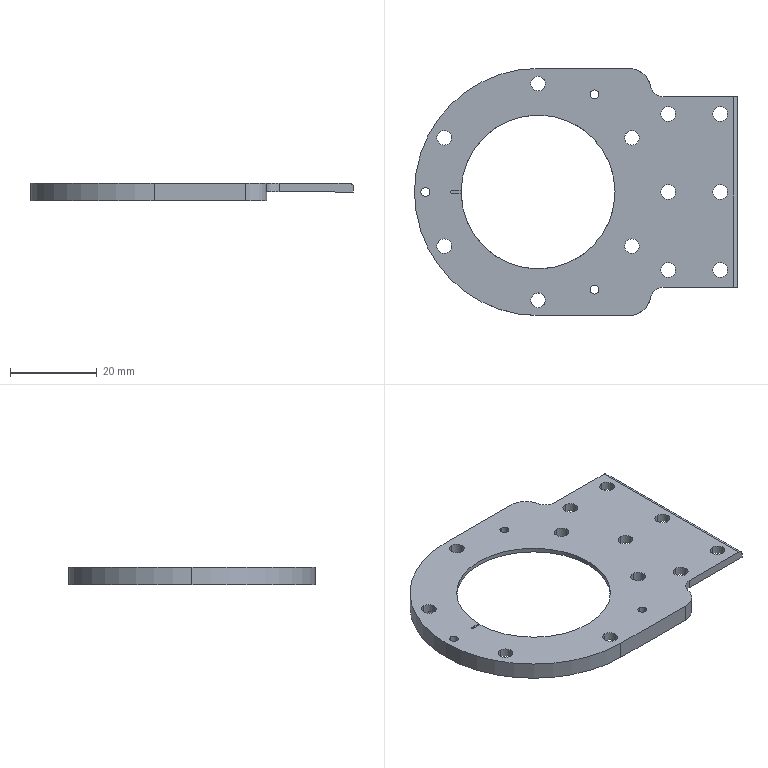NC program | NX | posted with a generic post | part box 74.5 x 57 x 4 mm
Lines 1 to 1634 of 1908, first 1478 of 1622 lines:
N10 G17 G21 G94 G90
(FLOOR_WALL_COPY , TOOL : D80)
N12 T19 M6
N14 G54
N16 G17 G0 G90 X-43. Y0. S5000 M3
N18 G43 Z30. H19
N20 Z3.
N22 G94 G1 Z0. F1200.
N24 X-40.
N26 X114.5
N28 X117.5
N30 Z3.
N32 G0 Z30.
N34 M5
(FLOOR_WALL_1 , TOOL : D4)
N36 T11 M6
N38 G54
N40 G17 G0 G90 X-3.5 Y-1.097 S9500 M3
N42 G43 Z30. H11
N44 Z0.62
N46 G94 G1 Z-0.38 F1000.
N48 X-2.2 Y-0.346
N50 G3 X-2. Y0. R0.4
N52 G1 Y24. F2500.
N54 X17.142
N56 G3 X17.95 Y24.411 R1.
N58 G1 X17.958 Y24.405
N60 G3 X17.9 Y23.5 R7.1
N62 G1 Y-23.5
N64 G3 X17.958 Y-24.405 R7.1
N66 G1 X17.95 Y-24.411
N68 G3 X17.142 Y-24. R1.
N70 G1 X-2.
N72 Y0.
N74 X0.4
N76 Y21.6
N78 X15.5
N80 Y-21.6
N82 X0.4
N84 Y0.
N86 X2.8
N88 Y19.2
N90 X13.1
N92 Y-19.2
N94 X2.8
N96 Y0.
N98 X5.2
N100 Y16.8
N102 X10.7
N104 Y-16.8
N106 X5.2
N108 Y0.
N110 X7.6
N112 Y14.4
N114 X8.3
N116 Y-14.4
N118 X7.6
N120 Y0.
N122 G3 X7.4 Y0.346 R0.4
N124 G1 Z0.62
N126 G0 X-3.5 Y-1.097 Z0.24
N128 G1 Z-0.76 F1000.
N130 X-2.2 Y-0.346
N132 G3 X-2. Y0. R0.4
N134 G1 Y24. F2500.
N136 X17.142
N138 G3 X17.95 Y24.411 R1.
N140 G1 X17.958 Y24.405
N142 G3 X17.9 Y23.5 R7.1
N144 G1 Y-23.5
N146 G3 X17.958 Y-24.405 R7.1
N148 G1 X17.95 Y-24.411
N150 G3 X17.142 Y-24. R1.
N152 G1 X-2.
N154 Y0.
N156 X0.4
N158 Y21.6
N160 X15.5
N162 Y-21.6
N164 X0.4
N166 Y0.
N168 X2.8
N170 Y19.2
N172 X13.1
N174 Y-19.2
N176 X2.8
N178 Y0.
N180 X5.2
N182 Y16.8
N184 X10.7
N186 Y-16.8
N188 X5.2
N190 Y0.
N192 X7.6
N194 Y14.4
N196 X8.3
N198 Y-14.4
N200 X7.6
N202 Y0.
N204 G3 X7.4 Y0.346 R0.4
N206 G1 Z0.24
N208 G0 X-3.5 Y-1.097 Z-0.14
N210 G1 Z-1.14 F1000.
N212 X-2.2 Y-0.346
N214 G3 X-2. Y0. R0.4
N216 G1 Y24. F2500.
N218 X17.142
N220 G3 X17.95 Y24.411 R1.
N222 G1 X17.958 Y24.405
N224 G3 X17.9 Y23.5 R7.1
N226 G1 Y-23.5
N228 G3 X17.958 Y-24.405 R7.1
N230 G1 X17.95 Y-24.411
N232 G3 X17.142 Y-24. R1.
N234 G1 X-2.
N236 Y0.
N238 X0.4
N240 Y21.6
N242 X15.5
N244 Y-21.6
N246 X0.4
N248 Y0.
N250 X2.8
N252 Y19.2
N254 X13.1
N256 Y-19.2
N258 X2.8
N260 Y0.
N262 X5.2
N264 Y16.8
N266 X10.7
N268 Y-16.8
N270 X5.2
N272 Y0.
N274 X7.6
N276 Y14.4
N278 X8.3
N280 Y-14.4
N282 X7.6
N284 Y0.
N286 G3 X7.4 Y0.346 R0.4
N288 G1 Z-0.14
N290 G0 X-3.5 Y-1.097 Z-0.52
N292 G1 Z-1.52 F1000.
N294 X-2.2 Y-0.346
N296 G3 X-2. Y0. R0.4
N298 G1 Y24. F2500.
N300 X17.142
N302 G3 X17.95 Y24.411 R1.
N304 G1 X17.958 Y24.405
N306 G3 X17.9 Y23.5 R7.1
N308 G1 Y-23.5
N310 G3 X17.958 Y-24.405 R7.1
N312 G1 X17.95 Y-24.411
N314 G3 X17.142 Y-24. R1.
N316 G1 X-2.
N318 Y0.
N320 X0.4
N322 Y21.6
N324 X15.5
N326 Y-21.6
N328 X0.4
N330 Y0.
N332 X2.8
N334 Y19.2
N336 X13.1
N338 Y-19.2
N340 X2.8
N342 Y0.
N344 X5.2
N346 Y16.8
N348 X10.7
N350 Y-16.8
N352 X5.2
N354 Y0.
N356 X7.6
N358 Y14.4
N360 X8.3
N362 Y-14.4
N364 X7.6
N366 Y0.
N368 G3 X7.4 Y0.346 R0.4
N370 G1 Z-0.52
N372 G0 X-3.5 Y-1.097 Z-0.9
N374 G1 Z-1.9 F1000.
N376 X-2.2 Y-0.346
N378 G3 X-2. Y0. R0.4
N380 G1 Y24. F2500.
N382 X17.142
N384 G3 X17.95 Y24.411 R1.
N386 G1 X17.958 Y24.405
N388 G3 X17.9 Y23.5 R7.1
N390 G1 Y-23.5
N392 G3 X17.958 Y-24.405 R7.1
N394 G1 X17.95 Y-24.411
N396 G3 X17.142 Y-24. R1.
N398 G1 X-2.
N400 Y0.
N402 X0.4
N404 Y21.6
N406 X15.5
N408 Y-21.6
N410 X0.4
N412 Y0.
N414 X2.8
N416 Y19.2
N418 X13.1
N420 Y-19.2
N422 X2.8
N424 Y0.
N426 X5.2
N428 Y16.8
N430 X10.7
N432 Y-16.8
N434 X5.2
N436 Y0.
N438 X7.6
N440 Y14.4
N442 X8.3
N444 Y-14.4
N446 X7.6
N448 Y0.
N450 G3 X7.4 Y0.346 R0.4
N452 G1 Z-0.9
N454 G0 Z30.
(FLOOR_WALL_1_COPY , TOOL : D4)
N456 X47.556 Y-21.217
N458 Z0.62
N460 G1 Z-0.38 F700.
N462 G3 X47.938 Y-21.336 R0.4
N464 X46. Y-22.707 R3.1 F2500.
N466 X43.709 Y-21.277 R3.1
N468 G2 X28.719 Y-12.623 R21.4
N470 G3 X26.335 Y-11.353 R3.1
N472 X26.428 Y-8.654 R3.1
N474 G2 X26.428 Y8.654 R21.4
N476 G3 X26.335 Y11.353 R3.1
N478 X28.719 Y12.623 R3.1
N480 G2 X43.709 Y21.277 R21.4
N482 G3 X46. Y22.707 R3.1
N484 X48.291 Y21.277 R3.1
N486 G2 X63.281 Y12.623 R21.4
N488 G3 X65.665 Y11.353 R3.1
N490 X65.572 Y8.654 R3.1
N492 G2 X65.572 Y-8.654 R21.4
N494 G3 X65.665 Y-11.353 R3.1
N496 X63.281 Y-12.623 R3.1
N498 G2 X48.291 Y-21.277 R21.4
N500 G3 X47.938 Y-21.336 R3.1
N502 G1 X47.407 Y-18.995
N504 G3 X46. Y-19.525 R5.5
N506 X43.966 Y-18.891 R5.5
N508 G2 X30.657 Y-11.207 R19.
N510 G3 X29.091 Y-9.762 R5.5
N512 X28.623 Y-7.684 R5.5
N514 G2 X28.623 Y7.684 R19.
N516 G3 X29.091 Y9.762 R5.5
N518 X30.657 Y11.207 R5.5
N520 G2 X43.966 Y18.891 R19.
N522 G3 X46. Y19.525 R5.5
N524 X48.034 Y18.891 R5.5
N526 G2 X61.343 Y11.207 R19.
N528 G3 X62.909 Y9.762 R5.5
N530 X63.377 Y7.684 R5.5
N532 G2 X63.377 Y-7.684 R19.
N534 G3 X62.909 Y-9.762 R5.5
N536 X61.343 Y-11.207 R5.5
N538 G2 X48.034 Y-18.891 R19.
N540 G3 X47.407 Y-18.995 R5.5
N542 G1 X46.877 Y-16.655
N544 G3 X46. Y-16.907 R7.9
N546 X44.223 Y-16.505 R7.9
N548 G2 X32.595 Y-9.791 R16.6
N550 G3 X31.358 Y-8.454 R7.9
N552 X30.818 Y-6.713 R7.9
N554 G2 X30.818 Y6.713 R16.6
N556 G3 X31.358 Y8.454 R7.9
N558 X32.595 Y9.791 R7.9
N560 G2 X44.223 Y16.505 R16.6
N562 G3 X46. Y16.907 R7.9
N564 X47.777 Y16.505 R7.9
N566 G2 X59.405 Y9.791 R16.6
N568 G3 X60.642 Y8.454 R7.9
N570 X61.182 Y6.713 R7.9
N572 G2 X61.182 Y-6.713 R16.6
N574 G3 X60.642 Y-8.454 R7.9
N576 X59.405 Y-9.791 R7.9
N578 G2 X47.777 Y-16.505 R16.6
N580 G3 X46.877 Y-16.655 R7.9
N582 X46.583 Y-16.926 R0.4
N584 G1 Z0.62
N586 G0 X47.556 Y-21.217 Z0.24
N588 G1 Z-0.76 F700.
N590 G3 X47.938 Y-21.336 R0.4
N592 X46. Y-22.707 R3.1 F2500.
N594 X43.709 Y-21.277 R3.1
N596 G2 X28.719 Y-12.623 R21.4
N598 G3 X26.335 Y-11.353 R3.1
N600 X26.428 Y-8.654 R3.1
N602 G2 X26.428 Y8.654 R21.4
N604 G3 X26.335 Y11.353 R3.1
N606 X28.719 Y12.623 R3.1
N608 G2 X43.709 Y21.277 R21.4
N610 G3 X46. Y22.707 R3.1
N612 X48.291 Y21.277 R3.1
N614 G2 X63.281 Y12.623 R21.4
N616 G3 X65.665 Y11.353 R3.1
N618 X65.572 Y8.654 R3.1
N620 G2 X65.572 Y-8.654 R21.4
N622 G3 X65.665 Y-11.353 R3.1
N624 X63.281 Y-12.623 R3.1
N626 G2 X48.291 Y-21.277 R21.4
N628 G3 X47.938 Y-21.336 R3.1
N630 G1 X47.407 Y-18.995
N632 G3 X46. Y-19.525 R5.5
N634 X43.966 Y-18.891 R5.5
N636 G2 X30.657 Y-11.207 R19.
N638 G3 X29.091 Y-9.762 R5.5
N640 X28.623 Y-7.684 R5.5
N642 G2 X28.623 Y7.684 R19.
N644 G3 X29.091 Y9.762 R5.5
N646 X30.657 Y11.207 R5.5
N648 G2 X43.966 Y18.891 R19.
N650 G3 X46. Y19.525 R5.5
N652 X48.034 Y18.891 R5.5
N654 G2 X61.343 Y11.207 R19.
N656 G3 X62.909 Y9.762 R5.5
N658 X63.377 Y7.684 R5.5
N660 G2 X63.377 Y-7.684 R19.
N662 G3 X62.909 Y-9.762 R5.5
N664 X61.343 Y-11.207 R5.5
N666 G2 X48.034 Y-18.891 R19.
N668 G3 X47.407 Y-18.995 R5.5
N670 G1 X46.877 Y-16.655
N672 G3 X46. Y-16.907 R7.9
N674 X44.223 Y-16.505 R7.9
N676 G2 X32.595 Y-9.791 R16.6
N678 G3 X31.358 Y-8.454 R7.9
N680 X30.818 Y-6.713 R7.9
N682 G2 X30.818 Y6.713 R16.6
N684 G3 X31.358 Y8.454 R7.9
N686 X32.595 Y9.791 R7.9
N688 G2 X44.223 Y16.505 R16.6
N690 G3 X46. Y16.907 R7.9
N692 X47.777 Y16.505 R7.9
N694 G2 X59.405 Y9.791 R16.6
N696 G3 X60.642 Y8.454 R7.9
N698 X61.182 Y6.713 R7.9
N700 G2 X61.182 Y-6.713 R16.6
N702 G3 X60.642 Y-8.454 R7.9
N704 X59.405 Y-9.791 R7.9
N706 G2 X47.777 Y-16.505 R16.6
N708 G3 X46.877 Y-16.655 R7.9
N710 X46.583 Y-16.926 R0.4
N712 G1 Z0.24
N714 G0 X47.556 Y-21.217 Z-0.14
N716 G1 Z-1.14 F700.
N718 G3 X47.938 Y-21.336 R0.4
N720 X46. Y-22.707 R3.1 F2500.
N722 X43.709 Y-21.277 R3.1
N724 G2 X28.719 Y-12.623 R21.4
N726 G3 X26.335 Y-11.353 R3.1
N728 X26.428 Y-8.654 R3.1
N730 G2 X26.428 Y8.654 R21.4
N732 G3 X26.335 Y11.353 R3.1
N734 X28.719 Y12.623 R3.1
N736 G2 X43.709 Y21.277 R21.4
N738 G3 X46. Y22.707 R3.1
N740 X48.291 Y21.277 R3.1
N742 G2 X63.281 Y12.623 R21.4
N744 G3 X65.665 Y11.353 R3.1
N746 X65.572 Y8.654 R3.1
N748 G2 X65.572 Y-8.654 R21.4
N750 G3 X65.665 Y-11.353 R3.1
N752 X63.281 Y-12.623 R3.1
N754 G2 X48.291 Y-21.277 R21.4
N756 G3 X47.938 Y-21.336 R3.1
N758 G1 X47.407 Y-18.995
N760 G3 X46. Y-19.525 R5.5
N762 X43.966 Y-18.891 R5.5
N764 G2 X30.657 Y-11.207 R19.
N766 G3 X29.091 Y-9.762 R5.5
N768 X28.623 Y-7.684 R5.5
N770 G2 X28.623 Y7.684 R19.
N772 G3 X29.091 Y9.762 R5.5
N774 X30.657 Y11.207 R5.5
N776 G2 X43.966 Y18.891 R19.
N778 G3 X46. Y19.525 R5.5
N780 X48.034 Y18.891 R5.5
N782 G2 X61.343 Y11.207 R19.
N784 G3 X62.909 Y9.762 R5.5
N786 X63.377 Y7.684 R5.5
N788 G2 X63.377 Y-7.684 R19.
N790 G3 X62.909 Y-9.762 R5.5
N792 X61.343 Y-11.207 R5.5
N794 G2 X48.034 Y-18.891 R19.
N796 G3 X47.407 Y-18.995 R5.5
N798 G1 X46.877 Y-16.655
N800 G3 X46. Y-16.907 R7.9
N802 X44.223 Y-16.505 R7.9
N804 G2 X32.595 Y-9.791 R16.6
N806 G3 X31.358 Y-8.454 R7.9
N808 X30.818 Y-6.713 R7.9
N810 G2 X30.818 Y6.713 R16.6
N812 G3 X31.358 Y8.454 R7.9
N814 X32.595 Y9.791 R7.9
N816 G2 X44.223 Y16.505 R16.6
N818 G3 X46. Y16.907 R7.9
N820 X47.777 Y16.505 R7.9
N822 G2 X59.405 Y9.791 R16.6
N824 G3 X60.642 Y8.454 R7.9
N826 X61.182 Y6.713 R7.9
N828 G2 X61.182 Y-6.713 R16.6
N830 G3 X60.642 Y-8.454 R7.9
N832 X59.405 Y-9.791 R7.9
N834 G2 X47.777 Y-16.505 R16.6
N836 G3 X46.877 Y-16.655 R7.9
N838 X46.583 Y-16.926 R0.4
N840 G1 Z-0.14
N842 G0 X47.556 Y-21.217 Z-0.52
N844 G1 Z-1.52 F700.
N846 G3 X47.938 Y-21.336 R0.4
N848 X46. Y-22.707 R3.1 F2500.
N850 X43.709 Y-21.277 R3.1
N852 G2 X28.719 Y-12.623 R21.4
N854 G3 X26.335 Y-11.353 R3.1
N856 X26.428 Y-8.654 R3.1
N858 G2 X26.428 Y8.654 R21.4
N860 G3 X26.335 Y11.353 R3.1
N862 X28.719 Y12.623 R3.1
N864 G2 X43.709 Y21.277 R21.4
N866 G3 X46. Y22.707 R3.1
N868 X48.291 Y21.277 R3.1
N870 G2 X63.281 Y12.623 R21.4
N872 G3 X65.665 Y11.353 R3.1
N874 X65.572 Y8.654 R3.1
N876 G2 X65.572 Y-8.654 R21.4
N878 G3 X65.665 Y-11.353 R3.1
N880 X63.281 Y-12.623 R3.1
N882 G2 X48.291 Y-21.277 R21.4
N884 G3 X47.938 Y-21.336 R3.1
N886 G1 X47.407 Y-18.995
N888 G3 X46. Y-19.525 R5.5
N890 X43.966 Y-18.891 R5.5
N892 G2 X30.657 Y-11.207 R19.
N894 G3 X29.091 Y-9.762 R5.5
N896 X28.623 Y-7.684 R5.5
N898 G2 X28.623 Y7.684 R19.
N900 G3 X29.091 Y9.762 R5.5
N902 X30.657 Y11.207 R5.5
N904 G2 X43.966 Y18.891 R19.
N906 G3 X46. Y19.525 R5.5
N908 X48.034 Y18.891 R5.5
N910 G2 X61.343 Y11.207 R19.
N912 G3 X62.909 Y9.762 R5.5
N914 X63.377 Y7.684 R5.5
N916 G2 X63.377 Y-7.684 R19.
N918 G3 X62.909 Y-9.762 R5.5
N920 X61.343 Y-11.207 R5.5
N922 G2 X48.034 Y-18.891 R19.
N924 G3 X47.407 Y-18.995 R5.5
N926 G1 X46.877 Y-16.655
N928 G3 X46. Y-16.907 R7.9
N930 X44.223 Y-16.505 R7.9
N932 G2 X32.595 Y-9.791 R16.6
N934 G3 X31.358 Y-8.454 R7.9
N936 X30.818 Y-6.713 R7.9
N938 G2 X30.818 Y6.713 R16.6
N940 G3 X31.358 Y8.454 R7.9
N942 X32.595 Y9.791 R7.9
N944 G2 X44.223 Y16.505 R16.6
N946 G3 X46. Y16.907 R7.9
N948 X47.777 Y16.505 R7.9
N950 G2 X59.405 Y9.791 R16.6
N952 G3 X60.642 Y8.454 R7.9
N954 X61.182 Y6.713 R7.9
N956 G2 X61.182 Y-6.713 R16.6
N958 G3 X60.642 Y-8.454 R7.9
N960 X59.405 Y-9.791 R7.9
N962 G2 X47.777 Y-16.505 R16.6
N964 G3 X46.877 Y-16.655 R7.9
N966 X46.583 Y-16.926 R0.4
N968 G1 Z-0.52
N970 G0 X47.556 Y-21.217 Z-0.9
N972 G1 Z-1.9 F700.
N974 G3 X47.938 Y-21.336 R0.4
N976 X46. Y-22.707 R3.1 F2500.
N978 X43.709 Y-21.277 R3.1
N980 G2 X28.719 Y-12.623 R21.4
N982 G3 X26.335 Y-11.353 R3.1
N984 X26.428 Y-8.654 R3.1
N986 G2 X26.428 Y8.654 R21.4
N988 G3 X26.335 Y11.353 R3.1
N990 X28.719 Y12.623 R3.1
N992 G2 X43.709 Y21.277 R21.4
N994 G3 X46. Y22.707 R3.1
N996 X48.291 Y21.277 R3.1
N998 G2 X63.281 Y12.623 R21.4
N1000 G3 X65.665 Y11.353 R3.1
N1002 X65.572 Y8.654 R3.1
N1004 G2 X65.572 Y-8.654 R21.4
N1006 G3 X65.665 Y-11.353 R3.1
N1008 X63.281 Y-12.623 R3.1
N1010 G2 X48.291 Y-21.277 R21.4
N1012 G3 X47.938 Y-21.336 R3.1
N1014 G1 X47.407 Y-18.995
N1016 G3 X46. Y-19.525 R5.5
N1018 X43.966 Y-18.891 R5.5
N1020 G2 X30.657 Y-11.207 R19.
N1022 G3 X29.091 Y-9.762 R5.5
N1024 X28.623 Y-7.684 R5.5
N1026 G2 X28.623 Y7.684 R19.
N1028 G3 X29.091 Y9.762 R5.5
N1030 X30.657 Y11.207 R5.5
N1032 G2 X43.966 Y18.891 R19.
N1034 G3 X46. Y19.525 R5.5
N1036 X48.034 Y18.891 R5.5
N1038 G2 X61.343 Y11.207 R19.
N1040 G3 X62.909 Y9.762 R5.5
N1042 X63.377 Y7.684 R5.5
N1044 G2 X63.377 Y-7.684 R19.
N1046 G3 X62.909 Y-9.762 R5.5
N1048 X61.343 Y-11.207 R5.5
N1050 G2 X48.034 Y-18.891 R19.
N1052 G3 X47.407 Y-18.995 R5.5
N1054 G1 X46.877 Y-16.655
N1056 G3 X46. Y-16.907 R7.9
N1058 X44.223 Y-16.505 R7.9
N1060 G2 X32.595 Y-9.791 R16.6
N1062 G3 X31.358 Y-8.454 R7.9
N1064 X30.818 Y-6.713 R7.9
N1066 G2 X30.818 Y6.713 R16.6
N1068 G3 X31.358 Y8.454 R7.9
N1070 X32.595 Y9.791 R7.9
N1072 G2 X44.223 Y16.505 R16.6
N1074 G3 X46. Y16.907 R7.9
N1076 X47.777 Y16.505 R7.9
N1078 G2 X59.405 Y9.791 R16.6
N1080 G3 X60.642 Y8.454 R7.9
N1082 X61.182 Y6.713 R7.9
N1084 G2 X61.182 Y-6.713 R16.6
N1086 G3 X60.642 Y-8.454 R7.9
N1088 X59.405 Y-9.791 R7.9
N1090 G2 X47.777 Y-16.505 R16.6
N1092 G3 X46.877 Y-16.655 R7.9
N1094 X46.583 Y-16.926 R0.4
N1096 G1 Z-0.9
N1098 G0 Z30.
(FLOOR_WALL_1_COPY_COPY , TOOL : D4)
N1100 X46.346 Y17.7
N1102 Z-1.3
N1104 G1 Z-2.3 F700.
N1106 G3 X46. Y17.9 R0.4
N1108 G2 X63.9 Y0. R17.9 F2500.
N1110 X46. Y17.9 R-17.9
N1112 G1 Y15.5
N1114 G2 X61.5 Y0. R15.5
N1116 X46. Y15.5 R-15.5
N1118 G3 X46.346 Y15.7 R0.4
N1120 G1 Z-1.3
N1122 G0 Y17.7 Z-1.6
N1124 G1 Z-2.6 F700.
N1126 G3 X46. Y17.9 R0.4
N1128 G2 X63.9 Y0. R17.9 F2500.
N1130 X46. Y17.9 R-17.9
N1132 G1 Y15.5
N1134 G2 X61.5 Y0. R15.5
N1136 X46. Y15.5 R-15.5
N1138 G3 X46.346 Y15.7 R0.4
N1140 G1 Z-1.6
N1142 G0 Y17.7 Z-1.9
N1144 G1 Z-2.9 F700.
N1146 G3 X46. Y17.9 R0.4
N1148 G2 X63.9 Y0. R17.9 F2500.
N1150 X46. Y17.9 R-17.9
N1152 G1 Y15.5
N1154 G2 X61.5 Y0. R15.5
N1156 X46. Y15.5 R-15.5
N1158 G3 X46.346 Y15.7 R0.4
N1160 G1 Z-1.9
N1162 G0 Z30.
N1164 M5
(FLOOR_WALL_1_COPY_COPY_1 , TOOL : D3)
N1166 T16 M6
N1168 G54
N1170 G17 G0 G90 X67.44 Y12.382 S9500 M3
N1172 G43 Z30. H16
N1174 Z-0.9
N1176 G94 G1 X67.473 Y12.409 Z-0.911 F700.
N1178 X67.448 Y12.388 Z-0.92
N1180 X67.423 Y12.369 Z-0.928
N1182 X67.453 Y12.381 Z-0.937
N1184 X67.483 Y12.392 Z-0.945
N1186 X67.453 Y12.381 Z-0.954
N1188 X67.423 Y12.369 Z-0.962
N1190 X67.448 Y12.388 Z-0.971
N1192 X67.473 Y12.409 Z-0.979
N1194 X67.448 Y12.388 Z-0.988
N1196 X67.423 Y12.369 Z-0.996
N1198 X67.453 Y12.381 Z-1.005
N1200 X67.483 Y12.392 Z-1.013
N1202 X67.453 Y12.381 Z-1.022
N1204 X67.423 Y12.369 Z-1.03
N1206 X67.448 Y12.388 Z-1.039
N1208 X67.473 Y12.409 Z-1.047
N1210 X67.448 Y12.388 Z-1.056
N1212 X67.423 Y12.369 Z-1.064
N1214 X67.453 Y12.381 Z-1.073
N1216 X67.483 Y12.392 Z-1.081
N1218 X67.453 Y12.381 Z-1.09
N1220 X67.423 Y12.369 Z-1.098
N1222 X67.448 Y12.388 Z-1.107
N1224 X67.473 Y12.409 Z-1.115
N1226 X67.448 Y12.388 Z-1.124
N1228 X67.423 Y12.369 Z-1.132
N1230 X67.453 Y12.381 Z-1.141
N1232 X67.483 Y12.392 Z-1.149
N1234 X67.453 Y12.381 Z-1.158
N1236 X67.423 Y12.369 Z-1.166
N1238 X67.448 Y12.388 Z-1.175
N1240 X67.473 Y12.409 Z-1.183
N1242 X67.448 Y12.388 Z-1.192
N1244 X67.423 Y12.369 Z-1.2
N1246 X67.453 Y12.381 Z-1.209
N1248 X67.483 Y12.392 Z-1.217
N1250 X67.453 Y12.381 Z-1.226
N1252 X67.423 Y12.369 Z-1.234
N1254 X67.448 Y12.388 Z-1.243
N1256 X67.473 Y12.409 Z-1.251
N1258 X67.448 Y12.388 Z-1.26
N1260 X67.423 Y12.369 Z-1.268
N1262 X67.453 Y12.381 Z-1.277
N1264 X67.483 Y12.392 Z-1.285
N1266 X67.453 Y12.381 Z-1.294
N1268 X67.423 Y12.369 Z-1.302
N1270 X67.448 Y12.388 Z-1.311
N1272 X67.473 Y12.409 Z-1.32
N1274 X67.448 Y12.388 Z-1.328
N1276 X67.423 Y12.369 Z-1.337
N1278 X67.453 Y12.381 Z-1.345
N1280 X67.483 Y12.392 Z-1.354
N1282 X67.453 Y12.381 Z-1.362
N1284 X67.423 Y12.369 Z-1.371
N1286 X67.448 Y12.388 Z-1.379
N1288 X67.473 Y12.409 Z-1.388
N1290 X67.448 Y12.388 Z-1.396
N1292 X67.423 Y12.369 Z-1.405
N1294 X67.453 Y12.381 Z-1.413
N1296 X67.483 Y12.392 Z-1.422
N1298 X67.453 Y12.381 Z-1.43
N1300 X67.423 Y12.369 Z-1.439
N1302 X67.448 Y12.388 Z-1.447
N1304 X67.473 Y12.409 Z-1.456
N1306 X67.448 Y12.388 Z-1.464
N1308 X67.423 Y12.369 Z-1.473
N1310 X67.453 Y12.381 Z-1.481
N1312 X67.483 Y12.392 Z-1.49
N1314 X67.453 Y12.381 Z-1.498
N1316 X67.423 Y12.369 Z-1.507
N1318 X67.448 Y12.388 Z-1.515
N1320 X67.473 Y12.409 Z-1.524
N1322 X67.448 Y12.388 Z-1.532
N1324 X67.423 Y12.369 Z-1.541
N1326 X67.453 Y12.381 Z-1.549
N1328 X67.483 Y12.392 Z-1.558
N1330 X67.453 Y12.381 Z-1.566
N1332 X67.423 Y12.369 Z-1.575
N1334 X67.448 Y12.388 Z-1.583
N1336 X67.473 Y12.409 Z-1.592
N1338 X67.448 Y12.388 Z-1.6
N1340 X67.423 Y12.369 Z-1.609
N1342 X67.453 Y12.381 Z-1.617
N1344 X67.483 Y12.392 Z-1.626
N1346 X67.453 Y12.381 Z-1.634
N1348 X67.423 Y12.369 Z-1.643
N1350 X67.448 Y12.388 Z-1.651
N1352 X67.473 Y12.409 Z-1.66
N1354 X67.448 Y12.388 Z-1.668
N1356 X67.423 Y12.369 Z-1.677
N1358 X67.453 Y12.381 Z-1.685
N1360 X67.483 Y12.392 Z-1.694
N1362 X67.453 Y12.381 Z-1.702
N1364 X67.423 Y12.369 Z-1.711
N1366 X67.448 Y12.388 Z-1.719
N1368 X67.473 Y12.409 Z-1.728
N1370 X67.448 Y12.388 Z-1.736
N1372 X67.423 Y12.369 Z-1.745
N1374 X67.453 Y12.381 Z-1.753
N1376 X67.483 Y12.392 Z-1.762
N1378 X67.453 Y12.381 Z-1.77
N1380 X67.423 Y12.369 Z-1.779
N1382 X67.448 Y12.388 Z-1.787
N1384 X67.473 Y12.409 Z-1.796
N1386 X67.448 Y12.388 Z-1.804
N1388 X67.423 Y12.369 Z-1.813
N1390 X67.453 Y12.381 Z-1.821
N1392 X67.483 Y12.392 Z-1.83
N1394 X67.453 Y12.381 Z-1.838
N1396 X67.423 Y12.369 Z-1.847
N1398 X67.448 Y12.388 Z-1.855
N1400 X67.473 Y12.409 Z-1.864
N1402 X67.448 Y12.388 Z-1.872
N1404 X67.423 Y12.369 Z-1.881
N1406 X67.453 Y12.381 Z-1.889
N1408 X67.483 Y12.392 Z-1.898
N1410 X67.453 Y12.381 Z-1.906
N1412 X67.423 Y12.369 Z-1.915
N1414 X67.448 Y12.388 Z-1.923
N1416 X67.473 Y12.409 Z-1.932
N1418 X67.448 Y12.388 Z-1.94
N1420 X67.423 Y12.369 Z-1.949
N1422 X67.453 Y12.381 Z-1.957
N1424 X67.483 Y12.392 Z-1.966
N1426 X67.453 Y12.381 Z-1.974
N1428 X67.423 Y12.369 Z-1.983
N1430 X67.448 Y12.388 Z-1.991
N1432 X67.473 Y12.409 Z-2.
N1434 X67.423 Y12.369 F1200.
N1436 X67.483 Y12.392
N1438 Z-1.
N1440 G0 Z30.
N1442 X48.354 Y21.56
N1444 Z-1.
N1446 G1 Z-2. F700.
N1448 G3 X48.127 Y21.756 R0.3
N1450 X48.339 Y21.724 R2.65 F1200.
N1452 G2 X63.644 Y12.888 R21.85
N1454 G3 X66.768 Y11.99 R2.65
N1456 X65.983 Y8.836 R2.65
N1458 G2 X65.983 Y-8.836 R21.85
N1460 G3 X66.768 Y-11.99 R2.65
N1462 X63.644 Y-12.888 R2.65
N1464 G2 X48.339 Y-21.724 R21.85
N1466 G3 X46. Y-23.981 R2.65
N1468 X43.661 Y-21.724 R2.65
N1470 G2 X28.356 Y-12.888 R21.85
N1472 G3 X25.232 Y-11.99 R2.65
N1474 X26.017 Y-8.836 R2.65
N1476 G2 X26.017 Y8.836 R21.85
N1478 G3 X25.232 Y11.99 R2.65
N1480 X28.356 Y12.888 R2.65
N1482 G2 X43.661 Y21.724 R21.85
N1484 G3 X46. Y23.981 R2.65
N1486 X48.127 Y21.756 R2.65
N1488 G1 X47.789 Y19.988
N1490 G3 X48.146 Y19.935 R4.45
N1492 G2 X62.191 Y11.826 R20.05
N1494 G3 X63.982 Y10.382 R4.45
N1496 X64.337 Y8.108 R4.45
N1498 G2 X64.337 Y-8.108 R20.05
N1500 G3 X63.982 Y-10.382 R4.45
N1502 X62.191 Y-11.826 R4.45
N1504 G2 X48.146 Y-19.935 R20.05
N1506 G3 X46. Y-20.764 R4.45
N1508 X43.854 Y-19.935 R4.45
N1510 G2 X29.809 Y-11.826 R20.05
N1512 G3 X28.018 Y-10.382 R4.45
N1514 X27.663 Y-8.108 R4.45
N1516 G2 X27.663 Y8.108 R20.05
N1518 G3 X28.018 Y10.382 R4.45
N1520 X29.809 Y11.826 R4.45
N1522 G2 X43.854 Y19.935 R20.05
N1524 G3 X46. Y20.764 R4.45
N1526 X47.789 Y19.988 R4.45
N1528 G1 X47.452 Y18.22
N1530 G3 X47.954 Y18.145 R6.25
N1532 G2 X60.737 Y10.765 R18.25
N1534 G3 X62.183 Y9.343 R6.25
N1536 X62.691 Y7.381 R6.25
N1538 G2 X62.691 Y-7.381 R18.25
N1540 G3 X62.183 Y-9.343 R6.25
N1542 X60.737 Y-10.765 R6.25
N1544 G2 X47.954 Y-18.145 R18.25
N1546 G3 X46. Y-18.686 R6.25
N1548 X44.046 Y-18.145 R6.25
N1550 G2 X31.263 Y-10.765 R18.25
N1552 G3 X29.817 Y-9.343 R6.25
N1554 X29.309 Y-7.381 R6.25
N1556 G2 X29.309 Y7.38 R18.25
N1558 G3 X29.817 Y9.343 R6.25
N1560 X31.263 Y10.765 R6.25
N1562 G2 X44.046 Y18.145 R18.25
N1564 G3 X46. Y18.686 R6.25
N1566 X47.452 Y18.22 R6.25
N1568 G1 X47.115 Y16.452
N1570 G3 X47.761 Y16.355 R8.05
N1572 G2 X59.284 Y9.703 R16.45
N1574 G3 X60.505 Y8.374 R8.05
N1576 X61.045 Y6.653 R8.05
N1578 G2 X61.045 Y-6.653 R16.45
N1580 G3 X60.505 Y-8.374 R8.05
N1582 X59.284 Y-9.703 R8.05
N1584 G2 X47.761 Y-16.355 R16.45
N1586 G3 X46. Y-16.748 R8.05
N1588 X44.239 Y-16.355 R8.05
N1590 G2 X32.716 Y-9.703 R16.45
N1592 G3 X31.495 Y-8.374 R8.05
N1594 X30.955 Y-6.653 R8.05
N1596 G2 X30.955 Y6.652 R16.45
N1598 G3 X31.495 Y8.374 R8.05
N1600 X32.716 Y9.703 R8.05
N1602 G2 X44.239 Y16.355 R16.45
N1604 G3 X46. Y16.748 R8.05
N1606 X47.115 Y16.452 R8.05
N1608 G1 X46.778 Y14.683
N1610 G3 X47.568 Y14.566 R9.85
N1612 G2 X57.83 Y8.641 R14.65
N1614 G3 X58.873 Y7.432 R9.85
N1616 X59.399 Y5.925 R9.85
N1618 G2 X59.399 Y-5.925 R14.65
N1620 G3 X58.873 Y-7.432 R9.85
N1622 X57.83 Y-8.641 R9.85
N1624 G2 X47.568 Y-14.566 R14.65
N1626 G3 X46. Y-14.865 R9.85
N1628 X44.432 Y-14.566 R9.85
N1630 G2 X34.17 Y-8.641 R14.65
N1632 G3 X33.127 Y-7.432 R9.85
N1634 X32.601 Y-5.925 R9.85
N1636 G2 X32.601 Y5.924 R14.65
N1638 G3 X33.127 Y7.432 R9.85
N1640 X34.17 Y8.641 R9.85
N1642 G2 X44.432 Y14.566 R14.65
N1644 G3 X46. Y14.865 R9.85
N1646 X46.778 Y14.683 R9.85
N1648 X47.061 Y14.782 R0.3
N1650 G1 Z-1.
N1652 G0 X45.997 Y24.759 Z-0.9
N1654 G1 X45.99 Y24.8 Z-0.911 F700.
N1656 X45.995 Y24.769 Z-0.92
N1658 X46. Y24.738 Z-0.928
N1660 X46.005 Y24.769 Z-0.937
N1662 X46.01 Y24.8 Z-0.945
N1664 X46.005 Y24.769 Z-0.954
N1666 X46. Y24.738 Z-0.962
N1668 X45.995 Y24.769 Z-0.971
N1670 X45.99 Y24.8 Z-0.979
N1672 X45.995 Y24.769 Z-0.988
N1674 X46. Y24.738 Z-0.996
N1676 X46.005 Y24.769 Z-1.005
N1678 X46.01 Y24.8 Z-1.013
N1680 X46.005 Y24.769 Z-1.022
N1682 X46. Y24.738 Z-1.03
N1684 X45.995 Y24.769 Z-1.039
N1686 X45.99 Y24.8 Z-1.047
N1688 X45.995 Y24.769 Z-1.056
N1690 X46. Y24.738 Z-1.064
N1692 X46.005 Y24.769 Z-1.073
N1694 X46.01 Y24.8 Z-1.081
N1696 X46.005 Y24.769 Z-1.09
N1698 X46. Y24.738 Z-1.098
N1700 X45.995 Y24.769 Z-1.107
N1702 X45.99 Y24.8 Z-1.115
N1704 X45.995 Y24.769 Z-1.124
N1706 X46. Y24.738 Z-1.132
N1708 X46.005 Y24.769 Z-1.141
N1710 X46.01 Y24.8 Z-1.149
N1712 X46.005 Y24.769 Z-1.158
N1714 X46. Y24.738 Z-1.166
N1716 X45.995 Y24.769 Z-1.175
N1718 X45.99 Y24.8 Z-1.183
N1720 X45.995 Y24.769 Z-1.192
N1722 X46. Y24.738 Z-1.2
N1724 X46.005 Y24.769 Z-1.209
N1726 X46.01 Y24.8 Z-1.217
N1728 X46.005 Y24.769 Z-1.226
N1730 X46. Y24.738 Z-1.234
N1732 X45.995 Y24.769 Z-1.243
N1734 X45.99 Y24.8 Z-1.251
N1736 X45.995 Y24.769 Z-1.26
N1738 X46. Y24.738 Z-1.268
N1740 X46.005 Y24.769 Z-1.277
N1742 X46.01 Y24.8 Z-1.285
N1744 X46.005 Y24.769 Z-1.294
N1746 X46. Y24.738 Z-1.302
N1748 X45.995 Y24.769 Z-1.311
N1750 X45.99 Y24.8 Z-1.32
N1752 X45.995 Y24.769 Z-1.328
N1754 X46. Y24.738 Z-1.337
N1756 X46.005 Y24.769 Z-1.345
N1758 X46.01 Y24.8 Z-1.354
N1760 X46.005 Y24.769 Z-1.362
N1762 X46. Y24.738 Z-1.371
N1764 X45.995 Y24.769 Z-1.379
N1766 X45.99 Y24.8 Z-1.388
N1768 X45.995 Y24.769 Z-1.396
N1770 X46. Y24.738 Z-1.405
N1772 X46.005 Y24.769 Z-1.413
N1774 X46.01 Y24.8 Z-1.422
N1776 X46.005 Y24.769 Z-1.43
N1778 X46. Y24.738 Z-1.439
N1780 X45.995 Y24.769 Z-1.447
N1782 X45.99 Y24.8 Z-1.456
N1784 X45.995 Y24.769 Z-1.464
N1786 X46. Y24.738 Z-1.473
N1788 X46.005 Y24.769 Z-1.481
N1790 X46.01 Y24.8 Z-1.49
N1792 X46.005 Y24.769 Z-1.498
N1794 X46. Y24.738 Z-1.507
N1796 X45.995 Y24.769 Z-1.515
N1798 X45.99 Y24.8 Z-1.524
N1800 X45.995 Y24.769 Z-1.532
N1802 X46. Y24.738 Z-1.541
N1804 X46.005 Y24.769 Z-1.549
N1806 X46.01 Y24.8 Z-1.558
N1808 X46.005 Y24.769 Z-1.566
N1810 X46. Y24.738 Z-1.575
N1812 X45.995 Y24.769 Z-1.583
N1814 X45.99 Y24.8 Z-1.592
N1816 X45.995 Y24.769 Z-1.6
N1818 X46. Y24.738 Z-1.609
N1820 X46.005 Y24.769 Z-1.617
N1822 X46.01 Y24.8 Z-1.626
N1824 X46.005 Y24.769 Z-1.634
N1826 X46. Y24.738 Z-1.643
N1828 X45.995 Y24.769 Z-1.651
N1830 X45.99 Y24.8 Z-1.66
N1832 X45.995 Y24.769 Z-1.668
N1834 X46. Y24.738 Z-1.677
N1836 X46.005 Y24.769 Z-1.685
N1838 X46.01 Y24.8 Z-1.694
N1840 X46.005 Y24.769 Z-1.702
N1842 X46. Y24.738 Z-1.711
N1844 X45.995 Y24.769 Z-1.719
N1846 X45.99 Y24.8 Z-1.728
N1848 X45.995 Y24.769 Z-1.736
N1850 X46. Y24.738 Z-1.745
N1852 X46.005 Y24.769 Z-1.753
N1854 X46.01 Y24.8 Z-1.762
N1856 X46.005 Y24.769 Z-1.77
N1858 X46. Y24.738 Z-1.779
N1860 X45.995 Y24.769 Z-1.787
N1862 X45.99 Y24.8 Z-1.796
N1864 X45.995 Y24.769 Z-1.804
N1866 X46. Y24.738 Z-1.813
N1868 X46.005 Y24.769 Z-1.821
N1870 X46.01 Y24.8 Z-1.83
N1872 X46.005 Y24.769 Z-1.838
N1874 X46. Y24.738 Z-1.847
N1876 X45.995 Y24.769 Z-1.855
N1878 X45.99 Y24.8 Z-1.864
N1880 X45.995 Y24.769 Z-1.872
N1882 X46. Y24.738 Z-1.881
N1884 X46.005 Y24.769 Z-1.889
N1886 X46.01 Y24.8 Z-1.898
N1888 X46.005 Y24.769 Z-1.906
N1890 X46. Y24.738 Z-1.915
N1892 X45.995 Y24.769 Z-1.923
N1894 X45.99 Y24.8 Z-1.932
N1896 X45.995 Y24.769 Z-1.94
N1898 X46. Y24.738 Z-1.949
N1900 X46.005 Y24.769 Z-1.957
N1902 X46.01 Y24.8 Z-1.966
N1904 X46.005 Y24.769 Z-1.974
N1906 X46. Y24.738 Z-1.983
N1908 X45.995 Y24.769 Z-1.991
N1910 X45.99 Y24.8 Z-2.
N1912 X46. Y24.738 F1200.
N1914 X46.01 Y24.8
N1916 Z-1.
N1918 G0 Z30.
N1920 X24.557 Y12.377
N1922 Z-0.9
N1924 G1 X24.517 Y12.392 Z-0.911 F700.
N1926 X24.547 Y12.381 Z-0.92
N1928 X24.577 Y12.369 Z-0.928
N1930 X24.552 Y12.388 Z-0.937
N1932 X24.527 Y12.409 Z-0.945
N1934 X24.552 Y12.388 Z-0.954
N1936 X24.577 Y12.369 Z-0.962
N1938 X24.547 Y12.381 Z-0.971
N1940 X24.517 Y12.392 Z-0.979
N1942 X24.547 Y12.381 Z-0.988
N1944 X24.577 Y12.369 Z-0.996
N1946 X24.552 Y12.388 Z-1.005
N1948 X24.527 Y12.409 Z-1.013
N1950 X24.552 Y12.388 Z-1.022
N1952 X24.577 Y12.369 Z-1.03
N1954 X24.547 Y12.381 Z-1.039
N1956 X24.517 Y12.392 Z-1.047
N1958 X24.547 Y12.381 Z-1.056
N1960 X24.577 Y12.369 Z-1.064
N1962 X24.552 Y12.388 Z-1.073
N1964 X24.527 Y12.409 Z-1.081
N1966 X24.552 Y12.388 Z-1.09
N1968 X24.577 Y12.369 Z-1.098
N1970 X24.547 Y12.381 Z-1.107
N1972 X24.517 Y12.392 Z-1.115
N1974 X24.547 Y12.381 Z-1.124
N1976 X24.577 Y12.369 Z-1.132
N1978 X24.552 Y12.388 Z-1.141
N1980 X24.527 Y12.409 Z-1.149
N1982 X24.552 Y12.388 Z-1.158
N1984 X24.577 Y12.369 Z-1.166
N1986 X24.547 Y12.381 Z-1.175
N1988 X24.517 Y12.392 Z-1.183
N1990 X24.547 Y12.381 Z-1.192
N1992 X24.577 Y12.369 Z-1.2
N1994 X24.552 Y12.388 Z-1.209
N1996 X24.527 Y12.409 Z-1.217
N1998 X24.552 Y12.388 Z-1.226
N2000 X24.577 Y12.369 Z-1.234
N2002 X24.547 Y12.381 Z-1.243
N2004 X24.517 Y12.392 Z-1.251
N2006 X24.547 Y12.381 Z-1.26
N2008 X24.577 Y12.369 Z-1.268
N2010 X24.552 Y12.388 Z-1.277
N2012 X24.527 Y12.409 Z-1.285
N2014 X24.552 Y12.388 Z-1.294
N2016 X24.577 Y12.369 Z-1.302
N2018 X24.547 Y12.381 Z-1.311
N2020 X24.517 Y12.392 Z-1.32
N2022 X24.547 Y12.381 Z-1.328
N2024 X24.577 Y12.369 Z-1.337
N2026 X24.552 Y12.388 Z-1.345
N2028 X24.527 Y12.409 Z-1.354
N2030 X24.552 Y12.388 Z-1.362
N2032 X24.577 Y12.369 Z-1.371
N2034 X24.547 Y12.381 Z-1.379
N2036 X24.517 Y12.392 Z-1.388
N2038 X24.547 Y12.381 Z-1.396
N2040 X24.577 Y12.369 Z-1.405
N2042 X24.552 Y12.388 Z-1.413
N2044 X24.527 Y12.409 Z-1.422
N2046 X24.552 Y12.388 Z-1.43
N2048 X24.577 Y12.369 Z-1.439
N2050 X24.547 Y12.381 Z-1.447
N2052 X24.517 Y12.392 Z-1.456
N2054 X24.547 Y12.381 Z-1.464
N2056 X24.577 Y12.369 Z-1.473
N2058 X24.552 Y12.388 Z-1.481
N2060 X24.527 Y12.409 Z-1.49
N2062 X24.552 Y12.388 Z-1.498
N2064 X24.577 Y12.369 Z-1.507
N2066 X24.547 Y12.381 Z-1.515
N2068 X24.517 Y12.392 Z-1.524
N2070 X24.547 Y12.381 Z-1.532
N2072 X24.577 Y12.369 Z-1.541
N2074 X24.552 Y12.388 Z-1.549
N2076 X24.527 Y12.409 Z-1.558
N2078 X24.552 Y12.388 Z-1.566
N2080 X24.577 Y12.369 Z-1.575
N2082 X24.547 Y12.381 Z-1.583
N2084 X24.517 Y12.392 Z-1.592
N2086 X24.547 Y12.381 Z-1.6
N2088 X24.577 Y12.369 Z-1.609
N2090 X24.552 Y12.388 Z-1.617
N2092 X24.527 Y12.409 Z-1.626
N2094 X24.552 Y12.388 Z-1.634
N2096 X24.577 Y12.369 Z-1.643
N2098 X24.547 Y12.381 Z-1.651
N2100 X24.517 Y12.392 Z-1.66
N2102 X24.547 Y12.381 Z-1.668
N2104 X24.577 Y12.369 Z-1.677
N2106 X24.552 Y12.388 Z-1.685
N2108 X24.527 Y12.409 Z-1.694
N2110 X24.552 Y12.388 Z-1.702
N2112 X24.577 Y12.369 Z-1.711
N2114 X24.547 Y12.381 Z-1.719
N2116 X24.517 Y12.392 Z-1.728
N2118 X24.547 Y12.381 Z-1.736
N2120 X24.577 Y12.369 Z-1.745
N2122 X24.552 Y12.388 Z-1.753
N2124 X24.527 Y12.409 Z-1.762
N2126 X24.552 Y12.388 Z-1.77
N2128 X24.577 Y12.369 Z-1.779
N2130 X24.547 Y12.381 Z-1.787
N2132 X24.517 Y12.392 Z-1.796
N2134 X24.547 Y12.381 Z-1.804
N2136 X24.577 Y12.369 Z-1.813
N2138 X24.552 Y12.388 Z-1.821
N2140 X24.527 Y12.409 Z-1.83
N2142 X24.552 Y12.388 Z-1.838
N2144 X24.577 Y12.369 Z-1.847
N2146 X24.547 Y12.381 Z-1.855
N2148 X24.517 Y12.392 Z-1.864
N2150 X24.547 Y12.381 Z-1.872
N2152 X24.577 Y12.369 Z-1.881
N2154 X24.552 Y12.388 Z-1.889
N2156 X24.527 Y12.409 Z-1.898
N2158 X24.552 Y12.388 Z-1.906
N2160 X24.577 Y12.369 Z-1.915
N2162 X24.547 Y12.381 Z-1.923
N2164 X24.517 Y12.392 Z-1.932
N2166 X24.547 Y12.381 Z-1.94
N2168 X24.577 Y12.369 Z-1.949
N2170 X24.552 Y12.388 Z-1.957
N2172 X24.527 Y12.409 Z-1.966
N2174 X24.552 Y12.388 Z-1.974
N2176 X24.577 Y12.369 Z-1.983
N2178 X24.547 Y12.381 Z-1.991
N2180 X24.517 Y12.392 Z-2.
N2182 X24.577 Y12.369 F1200.
N2184 X24.527 Y12.409
N2186 Z-1.
N2188 G0 Z30.
N2190 X24.56 Y-12.382
N2192 Z-0.9
N2194 G1 X24.527 Y-12.409 Z-0.911 F700.
N2196 X24.552 Y-12.388 Z-0.92
N2198 X24.577 Y-12.369 Z-0.928
N2200 X24.547 Y-12.381 Z-0.937
N2202 X24.517 Y-12.392 Z-0.945
N2204 X24.547 Y-12.381 Z-0.954
N2206 X24.577 Y-12.369 Z-0.962
N2208 X24.552 Y-12.388 Z-0.971
N2210 X24.527 Y-12.409 Z-0.979
N2212 X24.552 Y-12.388 Z-0.988
N2214 X24.577 Y-12.369 Z-0.996
N2216 X24.547 Y-12.381 Z-1.005
N2218 X24.517 Y-12.392 Z-1.013
N2220 X24.547 Y-12.381 Z-1.022
N2222 X24.577 Y-12.369 Z-1.03
N2224 X24.552 Y-12.388 Z-1.039
N2226 X24.527 Y-12.409 Z-1.047
N2228 X24.552 Y-12.388 Z-1.056
N2230 X24.577 Y-12.369 Z-1.064
N2232 X24.547 Y-12.381 Z-1.073
N2234 X24.517 Y-12.392 Z-1.081
N2236 X24.547 Y-12.381 Z-1.09
N2238 X24.577 Y-12.369 Z-1.098
N2240 X24.552 Y-12.388 Z-1.107
N2242 X24.527 Y-12.409 Z-1.115
N2244 X24.552 Y-12.388 Z-1.124
N2246 X24.577 Y-12.369 Z-1.132
N2248 X24.547 Y-12.381 Z-1.141
N2250 X24.517 Y-12.392 Z-1.149
N2252 X24.547 Y-12.381 Z-1.158
N2254 X24.577 Y-12.369 Z-1.166
N2256 X24.552 Y-12.388 Z-1.175
N2258 X24.527 Y-12.409 Z-1.183
N2260 X24.552 Y-12.388 Z-1.192
N2262 X24.577 Y-12.369 Z-1.2
N2264 X24.547 Y-12.381 Z-1.209
N2266 X24.517 Y-12.392 Z-1.217
N2268 X24.547 Y-12.381 Z-1.226
N2270 X24.577 Y-12.369 Z-1.234
N2272 X24.552 Y-12.388 Z-1.243
N2274 X24.527 Y-12.409 Z-1.251
N2276 X24.552 Y-12.388 Z-1.26
N2278 X24.577 Y-12.369 Z-1.268
N2280 X24.547 Y-12.381 Z-1.277
N2282 X24.517 Y-12.392 Z-1.285
N2284 X24.547 Y-12.381 Z-1.294
N2286 X24.577 Y-12.369 Z-1.302
N2288 X24.552 Y-12.388 Z-1.311
N2290 X24.527 Y-12.409 Z-1.32
N2292 X24.552 Y-12.388 Z-1.328
N2294 X24.577 Y-12.369 Z-1.337
N2296 X24.547 Y-12.381 Z-1.345
N2298 X24.517 Y-12.392 Z-1.354
N2300 X24.547 Y-12.381 Z-1.362
N2302 X24.577 Y-12.369 Z-1.371
N2304 X24.552 Y-12.388 Z-1.379
N2306 X24.527 Y-12.409 Z-1.388
N2308 X24.552 Y-12.388 Z-1.396
N2310 X24.577 Y-12.369 Z-1.405
N2312 X24.547 Y-12.381 Z-1.413
N2314 X24.517 Y-12.392 Z-1.422
N2316 X24.547 Y-12.381 Z-1.43
N2318 X24.577 Y-12.369 Z-1.439
N2320 X24.552 Y-12.388 Z-1.447
N2322 X24.527 Y-12.409 Z-1.456
N2324 X24.552 Y-12.388 Z-1.464
N2326 X24.577 Y-12.369 Z-1.473
N2328 X24.547 Y-12.381 Z-1.481
N2330 X24.517 Y-12.392 Z-1.49
N2332 X24.547 Y-12.381 Z-1.498
N2334 X24.577 Y-12.369 Z-1.507
N2336 X24.552 Y-12.388 Z-1.515
N2338 X24.527 Y-12.409 Z-1.524
N2340 X24.552 Y-12.388 Z-1.532
N2342 X24.577 Y-12.369 Z-1.541
N2344 X24.547 Y-12.381 Z-1.549
N2346 X24.517 Y-12.392 Z-1.558
N2348 X24.547 Y-12.381 Z-1.566
N2350 X24.577 Y-12.369 Z-1.575
N2352 X24.552 Y-12.388 Z-1.583
N2354 X24.527 Y-12.409 Z-1.592
N2356 X24.552 Y-12.388 Z-1.6
N2358 X24.577 Y-12.369 Z-1.609
N2360 X24.547 Y-12.381 Z-1.617
N2362 X24.517 Y-12.392 Z-1.626
N2364 X24.547 Y-12.381 Z-1.634
N2366 X24.577 Y-12.369 Z-1.643
N2368 X24.552 Y-12.388 Z-1.651
N2370 X24.527 Y-12.409 Z-1.66
N2372 X24.552 Y-12.388 Z-1.668
N2374 X24.577 Y-12.369 Z-1.677
N2376 X24.547 Y-12.381 Z-1.685
N2378 X24.517 Y-12.392 Z-1.694
N2380 X24.547 Y-12.381 Z-1.702
N2382 X24.577 Y-12.369 Z-1.711
N2384 X24.552 Y-12.388 Z-1.719
N2386 X24.527 Y-12.409 Z-1.728
N2388 X24.552 Y-12.388 Z-1.736
N2390 X24.577 Y-12.369 Z-1.745
N2392 X24.547 Y-12.381 Z-1.753
N2394 X24.517 Y-12.392 Z-1.762
N2396 X24.547 Y-12.381 Z-1.77
N2398 X24.577 Y-12.369 Z-1.779
N2400 X24.552 Y-12.388 Z-1.787
N2402 X24.527 Y-12.409 Z-1.796
N2404 X24.552 Y-12.388 Z-1.804
N2406 X24.577 Y-12.369 Z-1.813
N2408 X24.547 Y-12.381 Z-1.821
N2410 X24.517 Y-12.392 Z-1.83
N2412 X24.547 Y-12.381 Z-1.838
N2414 X24.577 Y-12.369 Z-1.847
N2416 X24.552 Y-12.388 Z-1.855
N2418 X24.527 Y-12.409 Z-1.864
N2420 X24.552 Y-12.388 Z-1.872
N2422 X24.577 Y-12.369 Z-1.881
N2424 X24.547 Y-12.381 Z-1.889
N2426 X24.517 Y-12.392 Z-1.898
N2428 X24.547 Y-12.381 Z-1.906
N2430 X24.577 Y-12.369 Z-1.915
N2432 X24.552 Y-12.388 Z-1.923
N2434 X24.527 Y-12.409 Z-1.932
N2436 X24.552 Y-12.388 Z-1.94
N2438 X24.577 Y-12.369 Z-1.949
N2440 X24.547 Y-12.381 Z-1.957
N2442 X24.517 Y-12.392 Z-1.966
N2444 X24.547 Y-12.381 Z-1.974
N2446 X24.577 Y-12.369 Z-1.983
N2448 X24.552 Y-12.388 Z-1.991
N2450 X24.527 Y-12.409 Z-2.
N2452 X24.577 Y-12.369 F1200.
N2454 X24.517 Y-12.392
N2456 Z-1.
N2458 G0 Z30.
N2460 X46.003 Y-24.759
N2462 Z-0.9
N2464 G1 X46.01 Y-24.8 Z-0.911 F700.
N2466 X46.005 Y-24.769 Z-0.92
N2468 X46. Y-24.738 Z-0.928
N2470 X45.995 Y-24.769 Z-0.937
N2472 X45.99 Y-24.8 Z-0.945
N2474 X45.995 Y-24.769 Z-0.954
N2476 X46. Y-24.738 Z-0.962
N2478 X46.005 Y-24.769 Z-0.971
N2480 X46.01 Y-24.8 Z-0.979
N2482 X46.005 Y-24.769 Z-0.988
N2484 X46. Y-24.738 Z-0.996
N2486 X45.995 Y-24.769 Z-1.005
N2488 X45.99 Y-24.8 Z-1.013
N2490 X45.995 Y-24.769 Z-1.022
N2492 X46. Y-24.738 Z-1.03
N2494 X46.005 Y-24.769 Z-1.039
N2496 X46.01 Y-24.8 Z-1.047
N2498 X46.005 Y-24.769 Z-1.056
N2500 X46. Y-24.738 Z-1.064
N2502 X45.995 Y-24.769 Z-1.073
N2504 X45.99 Y-24.8 Z-1.081
N2506 X45.995 Y-24.769 Z-1.09
N2508 X46. Y-24.738 Z-1.098
N2510 X46.005 Y-24.769 Z-1.107
N2512 X46.01 Y-24.8 Z-1.115
N2514 X46.005 Y-24.769 Z-1.124
N2516 X46. Y-24.738 Z-1.132
N2518 X45.995 Y-24.769 Z-1.141
N2520 X45.99 Y-24.8 Z-1.149
N2522 X45.995 Y-24.769 Z-1.158
N2524 X46. Y-24.738 Z-1.166
N2526 X46.005 Y-24.769 Z-1.175
N2528 X46.01 Y-24.8 Z-1.183
N2530 X46.005 Y-24.769 Z-1.192
N2532 X46. Y-24.738 Z-1.2
N2534 X45.995 Y-24.769 Z-1.209
N2536 X45.99 Y-24.8 Z-1.217
N2538 X45.995 Y-24.769 Z-1.226
N2540 X46. Y-24.738 Z-1.234
N2542 X46.005 Y-24.769 Z-1.243
N2544 X46.01 Y-24.8 Z-1.251
N2546 X46.005 Y-24.769 Z-1.26
N2548 X46. Y-24.738 Z-1.268
N2550 X45.995 Y-24.769 Z-1.277
N2552 X45.99 Y-24.8 Z-1.285
N2554 X45.995 Y-24.769 Z-1.294
N2556 X46. Y-24.738 Z-1.302
N2558 X46.005 Y-24.769 Z-1.311
N2560 X46.01 Y-24.8 Z-1.32
N2562 X46.005 Y-24.769 Z-1.328
N2564 X46. Y-24.738 Z-1.337
N2566 X45.995 Y-24.769 Z-1.345
N2568 X45.99 Y-24.8 Z-1.354
N2570 X45.995 Y-24.769 Z-1.362
N2572 X46. Y-24.738 Z-1.371
N2574 X46.005 Y-24.769 Z-1.379
N2576 X46.01 Y-24.8 Z-1.388
N2578 X46.005 Y-24.769 Z-1.396
N2580 X46. Y-24.738 Z-1.405
N2582 X45.995 Y-24.769 Z-1.413
N2584 X45.99 Y-24.8 Z-1.422
N2586 X45.995 Y-24.769 Z-1.43
N2588 X46. Y-24.738 Z-1.439
N2590 X46.005 Y-24.769 Z-1.447
N2592 X46.01 Y-24.8 Z-1.456
N2594 X46.005 Y-24.769 Z-1.464
N2596 X46. Y-24.738 Z-1.473
N2598 X45.995 Y-24.769 Z-1.481
N2600 X45.99 Y-24.8 Z-1.49
N2602 X45.995 Y-24.769 Z-1.498
N2604 X46. Y-24.738 Z-1.507
N2606 X46.005 Y-24.769 Z-1.515
N2608 X46.01 Y-24.8 Z-1.524
N2610 X46.005 Y-24.769 Z-1.532
N2612 X46. Y-24.738 Z-1.541
N2614 X45.995 Y-24.769 Z-1.549
N2616 X45.99 Y-24.8 Z-1.558
N2618 X45.995 Y-24.769 Z-1.566
N2620 X46. Y-24.738 Z-1.575
N2622 X46.005 Y-24.769 Z-1.583
N2624 X46.01 Y-24.8 Z-1.592
N2626 X46.005 Y-24.769 Z-1.6
N2628 X46. Y-24.738 Z-1.609
N2630 X45.995 Y-24.769 Z-1.617
N2632 X45.99 Y-24.8 Z-1.626
N2634 X45.995 Y-24.769 Z-1.634
N2636 X46. Y-24.738 Z-1.643
N2638 X46.005 Y-24.769 Z-1.651
N2640 X46.01 Y-24.8 Z-1.66
N2642 X46.005 Y-24.769 Z-1.668
N2644 X46. Y-24.738 Z-1.677
N2646 X45.995 Y-24.769 Z-1.685
N2648 X45.99 Y-24.8 Z-1.694
N2650 X45.995 Y-24.769 Z-1.702
N2652 X46. Y-24.738 Z-1.711
N2654 X46.005 Y-24.769 Z-1.719
N2656 X46.01 Y-24.8 Z-1.728
N2658 X46.005 Y-24.769 Z-1.736
N2660 X46. Y-24.738 Z-1.745
N2662 X45.995 Y-24.769 Z-1.753
N2664 X45.99 Y-24.8 Z-1.762
N2666 X45.995 Y-24.769 Z-1.77
N2668 X46. Y-24.738 Z-1.779
N2670 X46.005 Y-24.769 Z-1.787
N2672 X46.01 Y-24.8 Z-1.796
N2674 X46.005 Y-24.769 Z-1.804
N2676 X46. Y-24.738 Z-1.813
N2678 X45.995 Y-24.769 Z-1.821
N2680 X45.99 Y-24.8 Z-1.83
N2682 X45.995 Y-24.769 Z-1.838
N2684 X46. Y-24.738 Z-1.847
N2686 X46.005 Y-24.769 Z-1.855
N2688 X46.01 Y-24.8 Z-1.864
N2690 X46.005 Y-24.769 Z-1.872
N2692 X46. Y-24.738 Z-1.881
N2694 X45.995 Y-24.769 Z-1.889
N2696 X45.99 Y-24.8 Z-1.898
N2698 X45.995 Y-24.769 Z-1.906
N2700 X46. Y-24.738 Z-1.915
N2702 X46.005 Y-24.769 Z-1.923
N2704 X46.01 Y-24.8 Z-1.932
N2706 X46.005 Y-24.769 Z-1.94
N2708 X46. Y-24.738 Z-1.949
N2710 X45.995 Y-24.769 Z-1.957
N2712 X45.99 Y-24.8 Z-1.966
N2714 X45.995 Y-24.769 Z-1.974
N2716 X46. Y-24.738 Z-1.983
N2718 X46.005 Y-24.769 Z-1.991
N2720 X46.01 Y-24.8 Z-2.
N2722 X46. Y-24.738 F1200.
N2724 X45.99 Y-24.8
N2726 Z-1.
N2728 G0 Z30.
N2730 X67.443 Y-12.377
N2732 Z-0.9
N2734 G1 X67.483 Y-12.392 Z-0.911 F700.
N2736 X67.453 Y-12.381 Z-0.92
N2738 X67.423 Y-12.369 Z-0.928
N2740 X67.448 Y-12.388 Z-0.937
N2742 X67.473 Y-12.409 Z-0.945
N2744 X67.448 Y-12.388 Z-0.954
N2746 X67.423 Y-12.369 Z-0.962
N2748 X67.453 Y-12.381 Z-0.971
N2750 X67.483 Y-12.392 Z-0.979
N2752 X67.453 Y-12.381 Z-0.988
N2754 X67.423 Y-12.369 Z-0.996
N2756 X67.448 Y-12.388 Z-1.005
N2758 X67.473 Y-12.409 Z-1.013
N2760 X67.448 Y-12.388 Z-1.022
N2762 X67.423 Y-12.369 Z-1.03
N2764 X67.453 Y-12.381 Z-1.039
N2766 X67.483 Y-12.392 Z-1.047
N2768 X67.453 Y-12.381 Z-1.056
N2770 X67.423 Y-12.369 Z-1.064
N2772 X67.448 Y-12.388 Z-1.073
N2774 X67.473 Y-12.409 Z-1.081
N2776 X67.448 Y-12.388 Z-1.09
N2778 X67.423 Y-12.369 Z-1.098
N2780 X67.453 Y-12.381 Z-1.107
N2782 X67.483 Y-12.392 Z-1.115
N2784 X67.453 Y-12.381 Z-1.124
N2786 X67.423 Y-12.369 Z-1.132
N2788 X67.448 Y-12.388 Z-1.141
N2790 X67.473 Y-12.409 Z-1.149
N2792 X67.448 Y-12.388 Z-1.158
N2794 X67.423 Y-12.369 Z-1.166
N2796 X67.453 Y-12.381 Z-1.175
N2798 X67.483 Y-12.392 Z-1.183
N2800 X67.453 Y-12.381 Z-1.192
N2802 X67.423 Y-12.369 Z-1.2
N2804 X67.448 Y-12.388 Z-1.209
N2806 X67.473 Y-12.409 Z-1.217
N2808 X67.448 Y-12.388 Z-1.226
N2810 X67.423 Y-12.369 Z-1.234
N2812 X67.453 Y-12.381 Z-1.243
N2814 X67.483 Y-12.392 Z-1.251
N2816 X67.453 Y-12.381 Z-1.26
N2818 X67.423 Y-12.369 Z-1.268
N2820 X67.448 Y-12.388 Z-1.277
N2822 X67.473 Y-12.409 Z-1.285
N2824 X67.448 Y-12.388 Z-1.294
N2826 X67.423 Y-12.369 Z-1.302
N2828 X67.453 Y-12.381 Z-1.311
N2830 X67.483 Y-12.392 Z-1.32
N2832 X67.453 Y-12.381 Z-1.328
N2834 X67.423 Y-12.369 Z-1.337
N2836 X67.448 Y-12.388 Z-1.345
N2838 X67.473 Y-12.409 Z-1.354
N2840 X67.448 Y-12.388 Z-1.362
N2842 X67.423 Y-12.369 Z-1.371
N2844 X67.453 Y-12.381 Z-1.379
N2846 X67.483 Y-12.392 Z-1.388
N2848 X67.453 Y-12.381 Z-1.396
N2850 X67.423 Y-12.369 Z-1.405
N2852 X67.448 Y-12.388 Z-1.413
N2854 X67.473 Y-12.409 Z-1.422
N2856 X67.448 Y-12.388 Z-1.43
N2858 X67.423 Y-12.369 Z-1.439
N2860 X67.453 Y-12.381 Z-1.447
N2862 X67.483 Y-12.392 Z-1.456
N2864 X67.453 Y-12.381 Z-1.464
N2866 X67.423 Y-12.369 Z-1.473
N2868 X67.448 Y-12.388 Z-1.481
N2870 X67.473 Y-12.409 Z-1.49
N2872 X67.448 Y-12.388 Z-1.498
N2874 X67.423 Y-12.369 Z-1.507
N2876 X67.453 Y-12.381 Z-1.515
N2878 X67.483 Y-12.392 Z-1.524
N2880 X67.453 Y-12.381 Z-1.532
N2882 X67.423 Y-12.369 Z-1.541
N2884 X67.448 Y-12.388 Z-1.549
N2886 X67.473 Y-12.409 Z-1.558
N2888 X67.448 Y-12.388 Z-1.566
N2890 X67.423 Y-12.369 Z-1.575
N2892 X67.453 Y-12.381 Z-1.583
N2894 X67.483 Y-12.392 Z-1.592
N2896 X67.453 Y-12.381 Z-1.6
N2898 X67.423 Y-12.369 Z-1.609
N2900 X67.448 Y-12.388 Z-1.617
N2902 X67.473 Y-12.409 Z-1.626
N2904 X67.448 Y-12.388 Z-1.634
N2906 X67.423 Y-12.369 Z-1.643
N2908 X67.453 Y-12.381 Z-1.651
N2910 X67.483 Y-12.392 Z-1.66
N2912 X67.453 Y-12.381 Z-1.668
N2914 X67.423 Y-12.369 Z-1.677
N2916 X67.448 Y-12.388 Z-1.685
N2918 X67.473 Y-12.409 Z-1.694
N2920 X67.448 Y-12.388 Z-1.702
N2922 X67.423 Y-12.369 Z-1.711
N2924 X67.453 Y-12.381 Z-1.719
N2926 X67.483 Y-12.392 Z-1.728
N2928 X67.453 Y-12.381 Z-1.736
N2930 X67.423 Y-12.369 Z-1.745
N2932 X67.448 Y-12.388 Z-1.753
N2934 X67.473 Y-12.409 Z-1.762
N2936 X67.448 Y-12.388 Z-1.77
N2938 X67.423 Y-12.369 Z-1.779
N2940 X67.453 Y-12.381 Z-1.787
N2942 X67.483 Y-12.392 Z-1.796
N2944 X67.453 Y-12.381 Z-1.804
N2946 X67.423 Y-12.369 Z-1.813
N2948 X67.448 Y-12.388 Z-1.821
N2950 X67.473 Y-12.409 Z-1.83
N2952 X67.448 Y-12.388 Z-1.838
N2954 X67.423 Y-12.369 Z-1.847